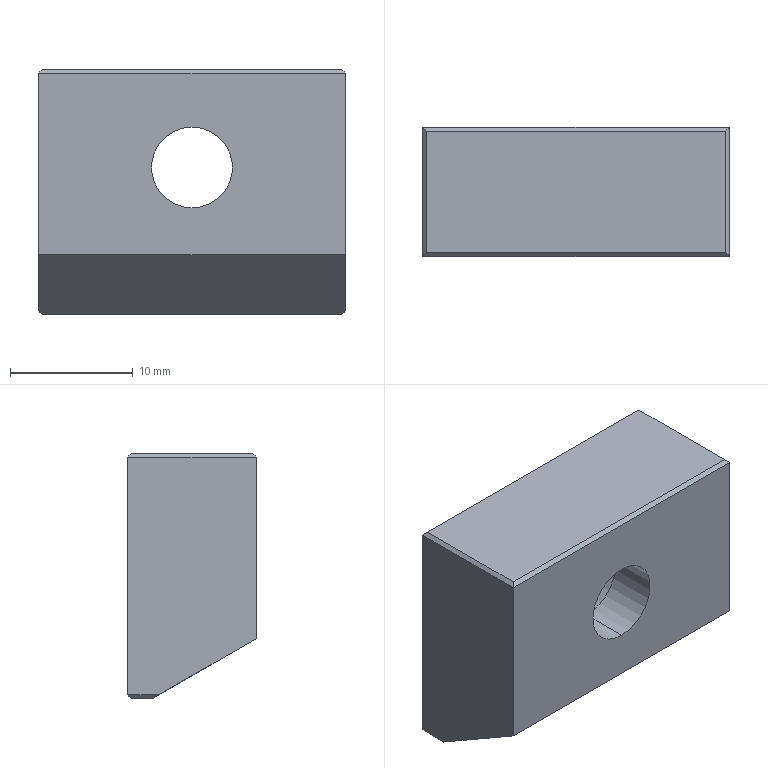Part | STEP file | P-0082091 | 1 solid | 19 faces | box 25 x 10.5 x 20 mm | volume 3970 mm3 | plane 15 | cylinder 4 | commonest cylinder face diameters 6.6 x2 11 x2
STEP:
#1=CARTESIAN_POINT('',(0.,0.,0.));
#2=DIRECTION('',(0.,0.,1.));
#3=DIRECTION('',(1.,0.,0.));
#4=AXIS2_PLACEMENT_3D('',#1,#2,#3);
#5=CARTESIAN_POINT('',(0.,-1.25,7.5));
#6=VERTEX_POINT('',#5);
#7=CARTESIAN_POINT('',(0.,5.25,7.5));
#8=VERTEX_POINT('',#7);
#9=CARTESIAN_POINT('',(0.,5.25,7.5));
#10=DIRECTION('',(0.,1.,0.));
#11=VECTOR('',#10,1.);
#12=LINE('',#9,#11);
#13=CARTESIAN_POINT('',(0.,5.25,2.));
#14=DIRECTION('',(0.,1.,0.));
#15=DIRECTION('',(0.,0.,1.));
#16=AXIS2_PLACEMENT_3D('',#13,#14,#15);
#17=CYLINDRICAL_SURFACE('',#16,5.5);
#18=CARTESIAN_POINT('',(6.283,0.));
#19=DIRECTION('',(0.,1.));
#20=VECTOR('',#19,1.);
#21=LINE('',#18,#20);
#22=(GEOMETRIC_REPRESENTATION_CONTEXT(2)PARAMETRIC_REPRESENTATION_CONTEXT()REPRESENTATION_CONTEXT('',''));
#23=DEFINITIONAL_REPRESENTATION('',(#21),#22);
#24=PCURVE('',#17,#23);
#25=CARTESIAN_POINT('',(0.,5.25,2.));
#26=DIRECTION('',(0.,1.,0.));
#27=DIRECTION('',(0.,0.,1.));
#28=AXIS2_PLACEMENT_3D('',#25,#26,#27);
#29=CYLINDRICAL_SURFACE('',#28,5.5);
#30=CARTESIAN_POINT('',(0.,0.));
#31=DIRECTION('',(0.,1.));
#32=VECTOR('',#31,1.);
#33=LINE('',#30,#32);
#34=(GEOMETRIC_REPRESENTATION_CONTEXT(2)PARAMETRIC_REPRESENTATION_CONTEXT()REPRESENTATION_CONTEXT('',''));
#35=DEFINITIONAL_REPRESENTATION('',(#33),#34);
#36=PCURVE('',#29,#35);
#37=SURFACE_CURVE('',#12,(#24,#36),.PCURVE_S1.);
#38=EDGE_CURVE('',#6,#8,#37,.T.);
#39=ORIENTED_EDGE('',*,*,#38,.T.);
#40=CARTESIAN_POINT('',(0.,5.25,-3.5));
#41=VERTEX_POINT('',#40);
#42=CARTESIAN_POINT('',(0.,5.25,2.));
#43=DIRECTION('',(0.,1.,0.));
#44=DIRECTION('',(0.,0.,1.));
#45=AXIS2_PLACEMENT_3D('',#42,#43,#44);
#46=CIRCLE('',#45,5.5);
#47=CARTESIAN_POINT('',(0.,0.));
#48=DIRECTION('',(1.,0.));
#49=VECTOR('',#48,1.);
#50=LINE('',#47,#49);
#51=(GEOMETRIC_REPRESENTATION_CONTEXT(2)PARAMETRIC_REPRESENTATION_CONTEXT()REPRESENTATION_CONTEXT('',''));
#52=DEFINITIONAL_REPRESENTATION('',(#50),#51);
#53=PCURVE('',#17,#52);
#54=CARTESIAN_POINT('',(12.5,5.25,10.));
#55=DIRECTION('',(0.,-1.,0.));
#56=DIRECTION('',(0.,0.,-1.));
#57=AXIS2_PLACEMENT_3D('',#54,#55,#56);
#58=PLANE('',#57);
#59=CARTESIAN_POINT('',(2.5,-12.5));
#60=CARTESIAN_POINT('',(2.5,-2.974));
#61=CARTESIAN_POINT('',(10.75,-7.737));
#62=CARTESIAN_POINT('',(19.,-12.5));
#63=CARTESIAN_POINT('',(10.75,-17.263));
#64=CARTESIAN_POINT('',(2.5,-22.026));
#65=CARTESIAN_POINT('',(2.5,-12.5));
#66=(BOUNDED_CURVE()B_SPLINE_CURVE(2,(#59,#60,#61,#62,#63,#64,#65),.UNSPECIFIED.,.T.,.F.)B_SPLINE_CURVE_WITH_KNOTS((1,2,2,2,2,1),(-2.094,0.,2.094,4.189,6.283,8.378),.UNSPECIFIED.)CURVE()GEOMETRIC_REPRESENTATION_ITEM()RATIONAL_B_SPLINE_CURVE((1.,0.5,1.,0.5,1.,0.5,1.))REPRESENTATION_ITEM(''));
#67=(GEOMETRIC_REPRESENTATION_CONTEXT(2)PARAMETRIC_REPRESENTATION_CONTEXT()REPRESENTATION_CONTEXT('',''));
#68=DEFINITIONAL_REPRESENTATION('',(#66),#67);
#69=PCURVE('',#58,#68);
#70=SURFACE_CURVE('',#46,(#53,#69),.PCURVE_S1.);
#71=EDGE_CURVE('',#41,#8,#70,.T.);
#72=ORIENTED_EDGE('',*,*,#71,.F.);
#73=CARTESIAN_POINT('',(0.,-1.25,-3.5));
#74=VERTEX_POINT('',#73);
#75=CARTESIAN_POINT('',(0.,5.25,-3.5));
#76=DIRECTION('',(0.,1.,0.));
#77=VECTOR('',#76,1.);
#78=LINE('',#75,#77);
#79=CARTESIAN_POINT('',(3.142,0.));
#80=DIRECTION('',(0.,1.));
#81=VECTOR('',#80,1.);
#82=LINE('',#79,#81);
#83=(GEOMETRIC_REPRESENTATION_CONTEXT(2)PARAMETRIC_REPRESENTATION_CONTEXT()REPRESENTATION_CONTEXT('',''));
#84=DEFINITIONAL_REPRESENTATION('',(#82),#83);
#85=PCURVE('',#17,#84);
#86=CARTESIAN_POINT('',(3.142,0.));
#87=DIRECTION('',(0.,1.));
#88=VECTOR('',#87,1.);
#89=LINE('',#86,#88);
#90=(GEOMETRIC_REPRESENTATION_CONTEXT(2)PARAMETRIC_REPRESENTATION_CONTEXT()REPRESENTATION_CONTEXT('',''));
#91=DEFINITIONAL_REPRESENTATION('',(#89),#90);
#92=PCURVE('',#29,#91);
#93=SURFACE_CURVE('',#78,(#85,#92),.PCURVE_S1.);
#94=EDGE_CURVE('',#74,#41,#93,.T.);
#95=ORIENTED_EDGE('',*,*,#94,.F.);
#96=CARTESIAN_POINT('',(0.,-1.25,2.));
#97=DIRECTION('',(0.,1.,0.));
#98=DIRECTION('',(0.,0.,1.));
#99=AXIS2_PLACEMENT_3D('',#96,#97,#98);
#100=CIRCLE('',#99,5.5);
#101=CARTESIAN_POINT('',(0.,-6.5));
#102=DIRECTION('',(1.,0.));
#103=VECTOR('',#102,1.);
#104=LINE('',#101,#103);
#105=(GEOMETRIC_REPRESENTATION_CONTEXT(2)PARAMETRIC_REPRESENTATION_CONTEXT()REPRESENTATION_CONTEXT('',''));
#106=DEFINITIONAL_REPRESENTATION('',(#104),#105);
#107=PCURVE('',#17,#106);
#108=CARTESIAN_POINT('',(3.3,-1.25,2.));
#109=DIRECTION('',(0.,-1.,0.));
#110=DIRECTION('',(0.,0.,-1.));
#111=AXIS2_PLACEMENT_3D('',#108,#109,#110);
#112=PLANE('',#111);
#113=CARTESIAN_POINT('',(-5.5,-3.3));
#114=CARTESIAN_POINT('',(-5.5,6.226));
#115=CARTESIAN_POINT('',(2.75,1.463));
#116=CARTESIAN_POINT('',(11.,-3.3));
#117=CARTESIAN_POINT('',(2.75,-8.063));
#118=CARTESIAN_POINT('',(-5.5,-12.826));
#119=CARTESIAN_POINT('',(-5.5,-3.3));
#120=(BOUNDED_CURVE()B_SPLINE_CURVE(2,(#113,#114,#115,#116,#117,#118,#119),.UNSPECIFIED.,.T.,.F.)B_SPLINE_CURVE_WITH_KNOTS((1,2,2,2,2,1),(-2.094,0.,2.094,4.189,6.283,8.378),.UNSPECIFIED.)CURVE()GEOMETRIC_REPRESENTATION_ITEM()RATIONAL_B_SPLINE_CURVE((1.,0.5,1.,0.5,1.,0.5,1.))REPRESENTATION_ITEM(''));
#121=(GEOMETRIC_REPRESENTATION_CONTEXT(2)PARAMETRIC_REPRESENTATION_CONTEXT()REPRESENTATION_CONTEXT('',''));
#122=DEFINITIONAL_REPRESENTATION('',(#120),#121);
#123=PCURVE('',#112,#122);
#124=SURFACE_CURVE('',#100,(#107,#123),.PCURVE_S1.);
#125=EDGE_CURVE('',#74,#6,#124,.T.);
#126=ORIENTED_EDGE('',*,*,#125,.T.);
#127=EDGE_LOOP('',(#39,#72,#95,#126));
#128=FACE_BOUND('',#127,.F.);
#129=ADVANCED_FACE('',(#128),#17,.F.);
#130=CARTESIAN_POINT('',(0.,-5.25,5.3));
#131=VERTEX_POINT('',#130);
#132=CARTESIAN_POINT('',(0.,-1.25,5.3));
#133=VERTEX_POINT('',#132);
#134=CARTESIAN_POINT('',(0.,5.25,5.3));
#135=DIRECTION('',(0.,1.,0.));
#136=VECTOR('',#135,1.);
#137=LINE('',#134,#136);
#138=CARTESIAN_POINT('',(0.,5.25,2.));
#139=DIRECTION('',(0.,1.,0.));
#140=DIRECTION('',(0.,0.,1.));
#141=AXIS2_PLACEMENT_3D('',#138,#139,#140);
#142=CYLINDRICAL_SURFACE('',#141,3.3);
#143=CARTESIAN_POINT('',(6.283,0.));
#144=DIRECTION('',(0.,1.));
#145=VECTOR('',#144,1.);
#146=LINE('',#143,#145);
#147=(GEOMETRIC_REPRESENTATION_CONTEXT(2)PARAMETRIC_REPRESENTATION_CONTEXT()REPRESENTATION_CONTEXT('',''));
#148=DEFINITIONAL_REPRESENTATION('',(#146),#147);
#149=PCURVE('',#142,#148);
#150=CARTESIAN_POINT('',(0.,5.25,2.));
#151=DIRECTION('',(0.,1.,0.));
#152=DIRECTION('',(0.,0.,1.));
#153=AXIS2_PLACEMENT_3D('',#150,#151,#152);
#154=CYLINDRICAL_SURFACE('',#153,3.3);
#155=CARTESIAN_POINT('',(0.,0.));
#156=DIRECTION('',(0.,1.));
#157=VECTOR('',#156,1.);
#158=LINE('',#155,#157);
#159=(GEOMETRIC_REPRESENTATION_CONTEXT(2)PARAMETRIC_REPRESENTATION_CONTEXT()REPRESENTATION_CONTEXT('',''));
#160=DEFINITIONAL_REPRESENTATION('',(#158),#159);
#161=PCURVE('',#154,#160);
#162=SURFACE_CURVE('',#137,(#149,#161),.PCURVE_S1.);
#163=EDGE_CURVE('',#131,#133,#162,.T.);
#164=ORIENTED_EDGE('',*,*,#163,.T.);
#165=CARTESIAN_POINT('',(0.,-1.25,-1.3));
#166=VERTEX_POINT('',#165);
#167=CARTESIAN_POINT('',(0.,-1.25,2.));
#168=DIRECTION('',(0.,1.,0.));
#169=DIRECTION('',(0.,0.,1.));
#170=AXIS2_PLACEMENT_3D('',#167,#168,#169);
#171=CIRCLE('',#170,3.3);
#172=CARTESIAN_POINT('',(0.,-6.5));
#173=DIRECTION('',(1.,0.));
#174=VECTOR('',#173,1.);
#175=LINE('',#172,#174);
#176=(GEOMETRIC_REPRESENTATION_CONTEXT(2)PARAMETRIC_REPRESENTATION_CONTEXT()REPRESENTATION_CONTEXT('',''));
#177=DEFINITIONAL_REPRESENTATION('',(#175),#176);
#178=PCURVE('',#142,#177);
#179=CARTESIAN_POINT('',(-3.3,-3.3));
#180=CARTESIAN_POINT('',(-3.3,2.416));
#181=CARTESIAN_POINT('',(1.65,-0.4421));
#182=CARTESIAN_POINT('',(6.6,-3.3));
#183=CARTESIAN_POINT('',(1.65,-6.158));
#184=CARTESIAN_POINT('',(-3.3,-9.016));
#185=CARTESIAN_POINT('',(-3.3,-3.3));
#186=(BOUNDED_CURVE()B_SPLINE_CURVE(2,(#179,#180,#181,#182,#183,#184,#185),.UNSPECIFIED.,.T.,.F.)B_SPLINE_CURVE_WITH_KNOTS((1,2,2,2,2,1),(-2.094,0.,2.094,4.189,6.283,8.378),.UNSPECIFIED.)CURVE()GEOMETRIC_REPRESENTATION_ITEM()RATIONAL_B_SPLINE_CURVE((1.,0.5,1.,0.5,1.,0.5,1.))REPRESENTATION_ITEM(''));
#187=(GEOMETRIC_REPRESENTATION_CONTEXT(2)PARAMETRIC_REPRESENTATION_CONTEXT()REPRESENTATION_CONTEXT('',''));
#188=DEFINITIONAL_REPRESENTATION('',(#186),#187);
#189=PCURVE('',#112,#188);
#190=SURFACE_CURVE('',#171,(#178,#189),.PCURVE_S1.);
#191=EDGE_CURVE('',#166,#133,#190,.T.);
#192=ORIENTED_EDGE('',*,*,#191,.F.);
#193=CARTESIAN_POINT('',(0.,-5.25,-1.3));
#194=VERTEX_POINT('',#193);
#195=CARTESIAN_POINT('',(0.,5.25,-1.3));
#196=DIRECTION('',(0.,1.,0.));
#197=VECTOR('',#196,1.);
#198=LINE('',#195,#197);
#199=CARTESIAN_POINT('',(3.142,0.));
#200=DIRECTION('',(0.,1.));
#201=VECTOR('',#200,1.);
#202=LINE('',#199,#201);
#203=(GEOMETRIC_REPRESENTATION_CONTEXT(2)PARAMETRIC_REPRESENTATION_CONTEXT()REPRESENTATION_CONTEXT('',''));
#204=DEFINITIONAL_REPRESENTATION('',(#202),#203);
#205=PCURVE('',#142,#204);
#206=CARTESIAN_POINT('',(3.142,0.));
#207=DIRECTION('',(0.,1.));
#208=VECTOR('',#207,1.);
#209=LINE('',#206,#208);
#210=(GEOMETRIC_REPRESENTATION_CONTEXT(2)PARAMETRIC_REPRESENTATION_CONTEXT()REPRESENTATION_CONTEXT('',''));
#211=DEFINITIONAL_REPRESENTATION('',(#209),#210);
#212=PCURVE('',#154,#211);
#213=SURFACE_CURVE('',#198,(#205,#212),.PCURVE_S1.);
#214=EDGE_CURVE('',#194,#166,#213,.T.);
#215=ORIENTED_EDGE('',*,*,#214,.F.);
#216=CARTESIAN_POINT('',(0.,-5.25,2.));
#217=DIRECTION('',(0.,1.,0.));
#218=DIRECTION('',(0.,0.,1.));
#219=AXIS2_PLACEMENT_3D('',#216,#217,#218);
#220=CIRCLE('',#219,3.3);
#221=CARTESIAN_POINT('',(0.,-10.5));
#222=DIRECTION('',(1.,0.));
#223=VECTOR('',#222,1.);
#224=LINE('',#221,#223);
#225=(GEOMETRIC_REPRESENTATION_CONTEXT(2)PARAMETRIC_REPRESENTATION_CONTEXT()REPRESENTATION_CONTEXT('',''));
#226=DEFINITIONAL_REPRESENTATION('',(#224),#225);
#227=PCURVE('',#142,#226);
#228=CARTESIAN_POINT('',(12.5,-5.25,-5.1));
#229=DIRECTION('',(0.,1.,0.));
#230=DIRECTION('',(0.,0.,1.));
#231=AXIS2_PLACEMENT_3D('',#228,#229,#230);
#232=PLANE('',#231);
#233=CARTESIAN_POINT('',(7.1,-12.5));
#234=DIRECTION('',(1.,0.));
#235=AXIS2_PLACEMENT_2D('',#233,#234);
#236=CIRCLE('',#235,3.3);
#237=(GEOMETRIC_REPRESENTATION_CONTEXT(2)PARAMETRIC_REPRESENTATION_CONTEXT()REPRESENTATION_CONTEXT('',''));
#238=DEFINITIONAL_REPRESENTATION('',(#236),#237);
#239=PCURVE('',#232,#238);
#240=SURFACE_CURVE('',#220,(#227,#239),.PCURVE_S1.);
#241=EDGE_CURVE('',#194,#131,#240,.T.);
#242=ORIENTED_EDGE('',*,*,#241,.T.);
#243=EDGE_LOOP('',(#164,#192,#215,#242));
#244=FACE_BOUND('',#243,.F.);
#245=ADVANCED_FACE('',(#244),#142,.F.);
#246=CARTESIAN_POINT('',(0.,-5.25,2.));
#247=DIRECTION('',(0.,1.,0.));
#248=DIRECTION('',(0.,0.,1.));
#249=AXIS2_PLACEMENT_3D('',#246,#247,#248);
#250=CIRCLE('',#249,3.3);
#251=CARTESIAN_POINT('',(7.1,-12.5));
#252=DIRECTION('',(1.,0.));
#253=AXIS2_PLACEMENT_2D('',#251,#252);
#254=CIRCLE('',#253,3.3);
#255=(GEOMETRIC_REPRESENTATION_CONTEXT(2)PARAMETRIC_REPRESENTATION_CONTEXT()REPRESENTATION_CONTEXT('',''));
#256=DEFINITIONAL_REPRESENTATION('',(#254),#255);
#257=PCURVE('',#232,#256);
#258=CARTESIAN_POINT('',(0.,-10.5));
#259=DIRECTION('',(1.,0.));
#260=VECTOR('',#259,1.);
#261=LINE('',#258,#260);
#262=(GEOMETRIC_REPRESENTATION_CONTEXT(2)PARAMETRIC_REPRESENTATION_CONTEXT()REPRESENTATION_CONTEXT('',''));
#263=DEFINITIONAL_REPRESENTATION('',(#261),#262);
#264=PCURVE('',#154,#263);
#265=SURFACE_CURVE('',#250,(#257,#264),.PCURVE_S1.);
#266=EDGE_CURVE('',#131,#194,#265,.T.);
#267=ORIENTED_EDGE('',*,*,#266,.T.);
#268=ORIENTED_EDGE('',*,*,#241,.T.);
#269=EDGE_LOOP('',(#267,#268));
#270=FACE_BOUND('',#269,.T.);
#271=CARTESIAN_POINT('',(12.5,-5.25,9.7));
#272=VERTEX_POINT('',#271);
#273=CARTESIAN_POINT('',(12.5,-5.25,-5.1));
#274=VERTEX_POINT('',#273);
#275=CARTESIAN_POINT('',(12.5,-5.25,-5.1));
#276=DIRECTION('',(0.,0.,-1.));
#277=VECTOR('',#276,1.);
#278=LINE('',#275,#277);
#279=CARTESIAN_POINT('',(0.,0.));
#280=DIRECTION('',(-1.,0.));
#281=VECTOR('',#280,1.);
#282=LINE('',#279,#281);
#283=(GEOMETRIC_REPRESENTATION_CONTEXT(2)PARAMETRIC_REPRESENTATION_CONTEXT()REPRESENTATION_CONTEXT('',''));
#284=DEFINITIONAL_REPRESENTATION('',(#282),#283);
#285=PCURVE('',#232,#284);
#286=CARTESIAN_POINT('',(12.5,0.,0.));
#287=DIRECTION('',(-1.,0.,0.));
#288=DIRECTION('',(0.,0.,1.));
#289=AXIS2_PLACEMENT_3D('',#286,#287,#288);
#290=PLANE('',#289);
#291=CARTESIAN_POINT('',(-5.1,-5.25));
#292=DIRECTION('',(-1.,0.));
#293=VECTOR('',#292,1.);
#294=LINE('',#291,#293);
#295=(GEOMETRIC_REPRESENTATION_CONTEXT(2)PARAMETRIC_REPRESENTATION_CONTEXT()REPRESENTATION_CONTEXT('',''));
#296=DEFINITIONAL_REPRESENTATION('',(#294),#295);
#297=PCURVE('',#290,#296);
#298=SURFACE_CURVE('',#278,(#285,#297),.PCURVE_S1.);
#299=EDGE_CURVE('',#272,#274,#298,.T.);
#300=ORIENTED_EDGE('',*,*,#299,.F.);
#301=CARTESIAN_POINT('',(-12.5,-5.25,9.7));
#302=VERTEX_POINT('',#301);
#303=CARTESIAN_POINT('',(12.5,-5.25,9.7));
#304=DIRECTION('',(-1.,0.,0.));
#305=VECTOR('',#304,1.);
#306=LINE('',#303,#305);
#307=CARTESIAN_POINT('',(14.8,0.));
#308=DIRECTION('',(0.,-1.));
#309=VECTOR('',#308,1.);
#310=LINE('',#307,#309);
#311=(GEOMETRIC_REPRESENTATION_CONTEXT(2)PARAMETRIC_REPRESENTATION_CONTEXT()REPRESENTATION_CONTEXT('',''));
#312=DEFINITIONAL_REPRESENTATION('',(#310),#311);
#313=PCURVE('',#232,#312);
#314=CARTESIAN_POINT('',(12.5,-5.25,9.7));
#315=DIRECTION('',(0.,0.7071,-0.7071));
#316=DIRECTION('',(-1.,0.,0.));
#317=AXIS2_PLACEMENT_3D('',#314,#315,#316);
#318=PLANE('',#317);
#319=CARTESIAN_POINT('',(0.,0.));
#320=DIRECTION('',(1.,0.));
#321=VECTOR('',#320,1.);
#322=LINE('',#319,#321);
#323=(GEOMETRIC_REPRESENTATION_CONTEXT(2)PARAMETRIC_REPRESENTATION_CONTEXT()REPRESENTATION_CONTEXT('',''));
#324=DEFINITIONAL_REPRESENTATION('',(#322),#323);
#325=PCURVE('',#318,#324);
#326=SURFACE_CURVE('',#306,(#313,#325),.PCURVE_S1.);
#327=EDGE_CURVE('',#272,#302,#326,.T.);
#328=ORIENTED_EDGE('',*,*,#327,.T.);
#329=CARTESIAN_POINT('',(-12.5,-5.25,-5.1));
#330=VERTEX_POINT('',#329);
#331=CARTESIAN_POINT('',(-12.5,-5.25,-5.1));
#332=DIRECTION('',(0.,0.,-1.));
#333=VECTOR('',#332,1.);
#334=LINE('',#331,#333);
#335=CARTESIAN_POINT('',(0.,-25.));
#336=DIRECTION('',(-1.,0.));
#337=VECTOR('',#336,1.);
#338=LINE('',#335,#337);
#339=(GEOMETRIC_REPRESENTATION_CONTEXT(2)PARAMETRIC_REPRESENTATION_CONTEXT()REPRESENTATION_CONTEXT('',''));
#340=DEFINITIONAL_REPRESENTATION('',(#338),#339);
#341=PCURVE('',#232,#340);
#342=CARTESIAN_POINT('',(-12.5,0.,0.));
#343=DIRECTION('',(-1.,0.,0.));
#344=DIRECTION('',(0.,0.,1.));
#345=AXIS2_PLACEMENT_3D('',#342,#343,#344);
#346=PLANE('',#345);
#347=CARTESIAN_POINT('',(-5.1,-5.25));
#348=DIRECTION('',(-1.,0.));
#349=VECTOR('',#348,1.);
#350=LINE('',#347,#349);
#351=(GEOMETRIC_REPRESENTATION_CONTEXT(2)PARAMETRIC_REPRESENTATION_CONTEXT()REPRESENTATION_CONTEXT('',''));
#352=DEFINITIONAL_REPRESENTATION('',(#350),#351);
#353=PCURVE('',#346,#352);
#354=SURFACE_CURVE('',#334,(#341,#353),.PCURVE_S1.);
#355=EDGE_CURVE('',#302,#330,#354,.T.);
#356=ORIENTED_EDGE('',*,*,#355,.T.);
#357=CARTESIAN_POINT('',(12.5,-5.25,-5.1));
#358=DIRECTION('',(-1.,0.,0.));
#359=VECTOR('',#358,1.);
#360=LINE('',#357,#359);
#361=CARTESIAN_POINT('',(0.,0.));
#362=DIRECTION('',(0.,-1.));
#363=VECTOR('',#362,1.);
#364=LINE('',#361,#363);
#365=(GEOMETRIC_REPRESENTATION_CONTEXT(2)PARAMETRIC_REPRESENTATION_CONTEXT()REPRESENTATION_CONTEXT('',''));
#366=DEFINITIONAL_REPRESENTATION('',(#364),#365);
#367=PCURVE('',#232,#366);
#368=CARTESIAN_POINT('',(12.5,3.25,-10.));
#369=DIRECTION('',(0.,0.4994,0.8664));
#370=DIRECTION('',(0.,-0.8664,0.4994));
#371=AXIS2_PLACEMENT_3D('',#368,#369,#370);
#372=PLANE('',#371);
#373=CARTESIAN_POINT('',(9.811,0.));
#374=DIRECTION('',(0.,-1.));
#375=VECTOR('',#374,1.);
#376=LINE('',#373,#375);
#377=(GEOMETRIC_REPRESENTATION_CONTEXT(2)PARAMETRIC_REPRESENTATION_CONTEXT()REPRESENTATION_CONTEXT('',''));
#378=DEFINITIONAL_REPRESENTATION('',(#376),#377);
#379=PCURVE('',#372,#378);
#380=SURFACE_CURVE('',#360,(#367,#379),.PCURVE_S1.);
#381=EDGE_CURVE('',#274,#330,#380,.T.);
#382=ORIENTED_EDGE('',*,*,#381,.F.);
#383=EDGE_LOOP('',(#300,#328,#356,#382));
#384=FACE_BOUND('',#383,.T.);
#385=ADVANCED_FACE('',(#270,#384),#232,.F.);
#386=CARTESIAN_POINT('',(-12.5,2.73,-9.7));
#387=VERTEX_POINT('',#386);
#388=CARTESIAN_POINT('',(-12.5,3.25,-10.));
#389=DIRECTION('',(0.,0.8664,-0.4994));
#390=VECTOR('',#389,1.);
#391=LINE('',#388,#390);
#392=CARTESIAN_POINT('',(0.,-25.));
#393=DIRECTION('',(-1.,0.));
#394=VECTOR('',#393,1.);
#395=LINE('',#392,#394);
#396=(GEOMETRIC_REPRESENTATION_CONTEXT(2)PARAMETRIC_REPRESENTATION_CONTEXT()REPRESENTATION_CONTEXT('',''));
#397=DEFINITIONAL_REPRESENTATION('',(#395),#396);
#398=PCURVE('',#372,#397);
#399=CARTESIAN_POINT('',(-10.,3.25));
#400=DIRECTION('',(-0.4994,0.8664));
#401=VECTOR('',#400,1.);
#402=LINE('',#399,#401);
#403=(GEOMETRIC_REPRESENTATION_CONTEXT(2)PARAMETRIC_REPRESENTATION_CONTEXT()REPRESENTATION_CONTEXT('',''));
#404=DEFINITIONAL_REPRESENTATION('',(#402),#403);
#405=PCURVE('',#346,#404);
#406=SURFACE_CURVE('',#391,(#398,#405),.PCURVE_S1.);
#407=EDGE_CURVE('',#330,#387,#406,.T.);
#408=ORIENTED_EDGE('',*,*,#407,.T.);
#409=CARTESIAN_POINT('',(-12.2,3.25,-10.));
#410=VERTEX_POINT('',#409);
#411=CARTESIAN_POINT('',(-11.507,4.451,-10.693));
#412=DIRECTION('',(0.4468,0.7751,-0.4468));
#413=VECTOR('',#412,1.);
#414=LINE('',#411,#413);
#415=CARTESIAN_POINT('',(-1.387,-24.007));
#416=DIRECTION('',(-0.8946,0.4468));
#417=VECTOR('',#416,1.);
#418=LINE('',#415,#417);
#419=(GEOMETRIC_REPRESENTATION_CONTEXT(2)PARAMETRIC_REPRESENTATION_CONTEXT()REPRESENTATION_CONTEXT('',''));
#420=DEFINITIONAL_REPRESENTATION('',(#418),#419);
#421=PCURVE('',#372,#420);
#422=CARTESIAN_POINT('',(-12.2,5.25,-10.));
#423=DIRECTION('',(-0.7071,0.,-0.7071));
#424=DIRECTION('',(0.,-1.,0.));
#425=AXIS2_PLACEMENT_3D('',#422,#423,#424);
#426=PLANE('',#425);
#427=CARTESIAN_POINT('',(0.7985,-0.9795));
#428=DIRECTION('',(-0.7751,-0.6319));
#429=VECTOR('',#428,1.);
#430=LINE('',#427,#429);
#431=(GEOMETRIC_REPRESENTATION_CONTEXT(2)PARAMETRIC_REPRESENTATION_CONTEXT()REPRESENTATION_CONTEXT('',''));
#432=DEFINITIONAL_REPRESENTATION('',(#430),#431);
#433=PCURVE('',#426,#432);
#434=SURFACE_CURVE('',#414,(#421,#433),.PCURVE_S1.);
#435=EDGE_CURVE('',#387,#410,#434,.T.);
#436=ORIENTED_EDGE('',*,*,#435,.T.);
#437=CARTESIAN_POINT('',(12.2,3.25,-10.));
#438=VERTEX_POINT('',#437);
#439=CARTESIAN_POINT('',(12.5,3.25,-10.));
#440=DIRECTION('',(-1.,0.,0.));
#441=VECTOR('',#440,1.);
#442=LINE('',#439,#441);
#443=CARTESIAN_POINT('',(0.,0.));
#444=DIRECTION('',(0.,-1.));
#445=VECTOR('',#444,1.);
#446=LINE('',#443,#445);
#447=(GEOMETRIC_REPRESENTATION_CONTEXT(2)PARAMETRIC_REPRESENTATION_CONTEXT()REPRESENTATION_CONTEXT('',''));
#448=DEFINITIONAL_REPRESENTATION('',(#446),#447);
#449=PCURVE('',#372,#448);
#450=CARTESIAN_POINT('',(12.5,5.25,-10.));
#451=DIRECTION('',(0.,0.,1.));
#452=DIRECTION('',(1.,0.,0.));
#453=AXIS2_PLACEMENT_3D('',#450,#451,#452);
#454=PLANE('',#453);
#455=CARTESIAN_POINT('',(0.,-2.));
#456=DIRECTION('',(-1.,0.));
#457=VECTOR('',#456,1.);
#458=LINE('',#455,#457);
#459=(GEOMETRIC_REPRESENTATION_CONTEXT(2)PARAMETRIC_REPRESENTATION_CONTEXT()REPRESENTATION_CONTEXT('',''));
#460=DEFINITIONAL_REPRESENTATION('',(#458),#459);
#461=PCURVE('',#454,#460);
#462=SURFACE_CURVE('',#442,(#449,#461),.PCURVE_S1.);
#463=EDGE_CURVE('',#438,#410,#462,.T.);
#464=ORIENTED_EDGE('',*,*,#463,.F.);
#465=CARTESIAN_POINT('',(12.5,2.73,-9.7));
#466=VERTEX_POINT('',#465);
#467=CARTESIAN_POINT('',(13.445,1.09,-8.755));
#468=DIRECTION('',(0.4468,-0.7751,0.4468));
#469=VECTOR('',#468,1.);
#470=LINE('',#467,#469);
#471=CARTESIAN_POINT('',(2.493,0.9453));
#472=DIRECTION('',(0.8946,0.4468));
#473=VECTOR('',#472,1.);
#474=LINE('',#471,#473);
#475=(GEOMETRIC_REPRESENTATION_CONTEXT(2)PARAMETRIC_REPRESENTATION_CONTEXT()REPRESENTATION_CONTEXT('',''));
#476=DEFINITIONAL_REPRESENTATION('',(#474),#475);
#477=PCURVE('',#372,#476);
#478=CARTESIAN_POINT('',(12.5,0.,-9.7));
#479=DIRECTION('',(-0.7071,0.,0.7071));
#480=DIRECTION('',(0.,1.,0.));
#481=AXIS2_PLACEMENT_3D('',#478,#479,#480);
#482=PLANE('',#481);
#483=CARTESIAN_POINT('',(1.09,-1.337));
#484=DIRECTION('',(-0.7751,-0.6319));
#485=VECTOR('',#484,1.);
#486=LINE('',#483,#485);
#487=(GEOMETRIC_REPRESENTATION_CONTEXT(2)PARAMETRIC_REPRESENTATION_CONTEXT()REPRESENTATION_CONTEXT('',''));
#488=DEFINITIONAL_REPRESENTATION('',(#486),#487);
#489=PCURVE('',#482,#488);
#490=SURFACE_CURVE('',#470,(#477,#489),.PCURVE_S1.);
#491=EDGE_CURVE('',#438,#466,#490,.T.);
#492=ORIENTED_EDGE('',*,*,#491,.T.);
#493=CARTESIAN_POINT('',(12.5,3.25,-10.));
#494=DIRECTION('',(0.,0.8664,-0.4994));
#495=VECTOR('',#494,1.);
#496=LINE('',#493,#495);
#497=CARTESIAN_POINT('',(0.,0.));
#498=DIRECTION('',(-1.,0.));
#499=VECTOR('',#498,1.);
#500=LINE('',#497,#499);
#501=(GEOMETRIC_REPRESENTATION_CONTEXT(2)PARAMETRIC_REPRESENTATION_CONTEXT()REPRESENTATION_CONTEXT('',''));
#502=DEFINITIONAL_REPRESENTATION('',(#500),#501);
#503=PCURVE('',#372,#502);
#504=CARTESIAN_POINT('',(-10.,3.25));
#505=DIRECTION('',(-0.4994,0.8664));
#506=VECTOR('',#505,1.);
#507=LINE('',#504,#506);
#508=(GEOMETRIC_REPRESENTATION_CONTEXT(2)PARAMETRIC_REPRESENTATION_CONTEXT()REPRESENTATION_CONTEXT('',''));
#509=DEFINITIONAL_REPRESENTATION('',(#507),#508);
#510=PCURVE('',#290,#509);
#511=SURFACE_CURVE('',#496,(#503,#510),.PCURVE_S1.);
#512=EDGE_CURVE('',#274,#466,#511,.T.);
#513=ORIENTED_EDGE('',*,*,#512,.F.);
#514=ORIENTED_EDGE('',*,*,#381,.T.);
#515=EDGE_LOOP('',(#408,#436,#464,#492,#513,#514));
#516=FACE_BOUND('',#515,.T.);
#517=ADVANCED_FACE('',(#516),#372,.F.);
#518=ORIENTED_EDGE('',*,*,#463,.T.);
#519=CARTESIAN_POINT('',(-12.2,4.95,-10.));
#520=VERTEX_POINT('',#519);
#521=CARTESIAN_POINT('',(-12.2,5.25,-10.));
#522=DIRECTION('',(0.,1.,0.));
#523=VECTOR('',#522,1.);
#524=LINE('',#521,#523);
#525=CARTESIAN_POINT('',(-24.7,0.));
#526=DIRECTION('',(0.,1.));
#527=VECTOR('',#526,1.);
#528=LINE('',#525,#527);
#529=(GEOMETRIC_REPRESENTATION_CONTEXT(2)PARAMETRIC_REPRESENTATION_CONTEXT()REPRESENTATION_CONTEXT('',''));
#530=DEFINITIONAL_REPRESENTATION('',(#528),#529);
#531=PCURVE('',#454,#530);
#532=CARTESIAN_POINT('',(0.,0.));
#533=DIRECTION('',(-1.,0.));
#534=VECTOR('',#533,1.);
#535=LINE('',#532,#534);
#536=(GEOMETRIC_REPRESENTATION_CONTEXT(2)PARAMETRIC_REPRESENTATION_CONTEXT()REPRESENTATION_CONTEXT('',''));
#537=DEFINITIONAL_REPRESENTATION('',(#535),#536);
#538=PCURVE('',#426,#537);
#539=SURFACE_CURVE('',#524,(#531,#538),.PCURVE_S1.);
#540=EDGE_CURVE('',#410,#520,#539,.T.);
#541=ORIENTED_EDGE('',*,*,#540,.T.);
#542=CARTESIAN_POINT('',(12.2,4.95,-10.));
#543=VERTEX_POINT('',#542);
#544=CARTESIAN_POINT('',(12.5,4.95,-10.));
#545=DIRECTION('',(1.,0.,0.));
#546=VECTOR('',#545,1.);
#547=LINE('',#544,#546);
#548=CARTESIAN_POINT('',(0.,-0.3));
#549=DIRECTION('',(1.,0.));
#550=VECTOR('',#549,1.);
#551=LINE('',#548,#550);
#552=(GEOMETRIC_REPRESENTATION_CONTEXT(2)PARAMETRIC_REPRESENTATION_CONTEXT()REPRESENTATION_CONTEXT('',''));
#553=DEFINITIONAL_REPRESENTATION('',(#551),#552);
#554=PCURVE('',#454,#553);
#555=CARTESIAN_POINT('',(12.5,5.25,-9.7));
#556=DIRECTION('',(0.,-0.7071,0.7071));
#557=DIRECTION('',(-1.,0.,0.));
#558=AXIS2_PLACEMENT_3D('',#555,#556,#557);
#559=PLANE('',#558);
#560=CARTESIAN_POINT('',(0.,0.4243));
#561=DIRECTION('',(-1.,0.));
#562=VECTOR('',#561,1.);
#563=LINE('',#560,#562);
#564=(GEOMETRIC_REPRESENTATION_CONTEXT(2)PARAMETRIC_REPRESENTATION_CONTEXT()REPRESENTATION_CONTEXT('',''));
#565=DEFINITIONAL_REPRESENTATION('',(#563),#564);
#566=PCURVE('',#559,#565);
#567=SURFACE_CURVE('',#547,(#554,#566),.PCURVE_S1.);
#568=EDGE_CURVE('',#520,#543,#567,.T.);
#569=ORIENTED_EDGE('',*,*,#568,.T.);
#570=CARTESIAN_POINT('',(12.2,5.25,-10.));
#571=DIRECTION('',(0.,-1.,0.));
#572=VECTOR('',#571,1.);
#573=LINE('',#570,#572);
#574=CARTESIAN_POINT('',(-0.3,0.));
#575=DIRECTION('',(0.,-1.));
#576=VECTOR('',#575,1.);
#577=LINE('',#574,#576);
#578=(GEOMETRIC_REPRESENTATION_CONTEXT(2)PARAMETRIC_REPRESENTATION_CONTEXT()REPRESENTATION_CONTEXT('',''));
#579=DEFINITIONAL_REPRESENTATION('',(#577),#578);
#580=PCURVE('',#454,#579);
#581=CARTESIAN_POINT('',(5.25,0.4243));
#582=DIRECTION('',(-1.,0.));
#583=VECTOR('',#582,1.);
#584=LINE('',#581,#583);
#585=(GEOMETRIC_REPRESENTATION_CONTEXT(2)PARAMETRIC_REPRESENTATION_CONTEXT()REPRESENTATION_CONTEXT('',''));
#586=DEFINITIONAL_REPRESENTATION('',(#584),#585);
#587=PCURVE('',#482,#586);
#588=SURFACE_CURVE('',#573,(#580,#587),.PCURVE_S1.);
#589=EDGE_CURVE('',#543,#438,#588,.T.);
#590=ORIENTED_EDGE('',*,*,#589,.T.);
#591=EDGE_LOOP('',(#518,#541,#569,#590));
#592=FACE_BOUND('',#591,.T.);
#593=ADVANCED_FACE('',(#592),#454,.F.);
#594=CARTESIAN_POINT('',(0.,5.25,2.));
#595=DIRECTION('',(0.,1.,0.));
#596=DIRECTION('',(0.,0.,1.));
#597=AXIS2_PLACEMENT_3D('',#594,#595,#596);
#598=CIRCLE('',#597,5.5);
#599=CARTESIAN_POINT('',(2.5,-12.5));
#600=CARTESIAN_POINT('',(2.5,-2.974));
#601=CARTESIAN_POINT('',(10.75,-7.737));
#602=CARTESIAN_POINT('',(19.,-12.5));
#603=CARTESIAN_POINT('',(10.75,-17.263));
#604=CARTESIAN_POINT('',(2.5,-22.026));
#605=CARTESIAN_POINT('',(2.5,-12.5));
#606=(BOUNDED_CURVE()B_SPLINE_CURVE(2,(#599,#600,#601,#602,#603,#604,#605),.UNSPECIFIED.,.T.,.F.)B_SPLINE_CURVE_WITH_KNOTS((1,2,2,2,2,1),(-2.094,0.,2.094,4.189,6.283,8.378),.UNSPECIFIED.)CURVE()GEOMETRIC_REPRESENTATION_ITEM()RATIONAL_B_SPLINE_CURVE((1.,0.5,1.,0.5,1.,0.5,1.))REPRESENTATION_ITEM(''));
#607=(GEOMETRIC_REPRESENTATION_CONTEXT(2)PARAMETRIC_REPRESENTATION_CONTEXT()REPRESENTATION_CONTEXT('',''));
#608=DEFINITIONAL_REPRESENTATION('',(#606),#607);
#609=PCURVE('',#58,#608);
#610=CARTESIAN_POINT('',(0.,0.));
#611=DIRECTION('',(1.,0.));
#612=VECTOR('',#611,1.);
#613=LINE('',#610,#612);
#614=(GEOMETRIC_REPRESENTATION_CONTEXT(2)PARAMETRIC_REPRESENTATION_CONTEXT()REPRESENTATION_CONTEXT('',''));
#615=DEFINITIONAL_REPRESENTATION('',(#613),#614);
#616=PCURVE('',#29,#615);
#617=SURFACE_CURVE('',#598,(#609,#616),.PCURVE_S1.);
#618=EDGE_CURVE('',#8,#41,#617,.T.);
#619=ORIENTED_EDGE('',*,*,#618,.F.);
#620=ORIENTED_EDGE('',*,*,#71,.F.);
#621=EDGE_LOOP('',(#619,#620));
#622=FACE_BOUND('',#621,.T.);
#623=CARTESIAN_POINT('',(-12.5,5.25,-9.7));
#624=VERTEX_POINT('',#623);
#625=CARTESIAN_POINT('',(-12.5,5.25,9.7));
#626=VERTEX_POINT('',#625);
#627=CARTESIAN_POINT('',(-12.5,5.25,10.));
#628=DIRECTION('',(0.,0.,1.));
#629=VECTOR('',#628,1.);
#630=LINE('',#627,#629);
#631=CARTESIAN_POINT('',(0.,-25.));
#632=DIRECTION('',(-1.,0.));
#633=VECTOR('',#632,1.);
#634=LINE('',#631,#633);
#635=(GEOMETRIC_REPRESENTATION_CONTEXT(2)PARAMETRIC_REPRESENTATION_CONTEXT()REPRESENTATION_CONTEXT('',''));
#636=DEFINITIONAL_REPRESENTATION('',(#634),#635);
#637=PCURVE('',#58,#636);
#638=CARTESIAN_POINT('',(10.,5.25));
#639=DIRECTION('',(1.,0.));
#640=VECTOR('',#639,1.);
#641=LINE('',#638,#640);
#642=(GEOMETRIC_REPRESENTATION_CONTEXT(2)PARAMETRIC_REPRESENTATION_CONTEXT()REPRESENTATION_CONTEXT('',''));
#643=DEFINITIONAL_REPRESENTATION('',(#641),#642);
#644=PCURVE('',#346,#643);
#645=SURFACE_CURVE('',#630,(#637,#644),.PCURVE_S1.);
#646=EDGE_CURVE('',#624,#626,#645,.T.);
#647=ORIENTED_EDGE('',*,*,#646,.T.);
#648=CARTESIAN_POINT('',(12.5,5.25,9.7));
#649=VERTEX_POINT('',#648);
#650=CARTESIAN_POINT('',(12.5,5.25,9.7));
#651=DIRECTION('',(1.,0.,0.));
#652=VECTOR('',#651,1.);
#653=LINE('',#650,#652);
#654=CARTESIAN_POINT('',(0.3,0.));
#655=DIRECTION('',(0.,1.));
#656=VECTOR('',#655,1.);
#657=LINE('',#654,#656);
#658=(GEOMETRIC_REPRESENTATION_CONTEXT(2)PARAMETRIC_REPRESENTATION_CONTEXT()REPRESENTATION_CONTEXT('',''));
#659=DEFINITIONAL_REPRESENTATION('',(#657),#658);
#660=PCURVE('',#58,#659);
#661=CARTESIAN_POINT('',(12.5,4.95,10.));
#662=DIRECTION('',(0.,-0.7071,-0.7071));
#663=DIRECTION('',(-1.,0.,0.));
#664=AXIS2_PLACEMENT_3D('',#661,#662,#663);
#665=PLANE('',#664);
#666=CARTESIAN_POINT('',(0.,0.4243));
#667=DIRECTION('',(-1.,0.));
#668=VECTOR('',#667,1.);
#669=LINE('',#666,#668);
#670=(GEOMETRIC_REPRESENTATION_CONTEXT(2)PARAMETRIC_REPRESENTATION_CONTEXT()REPRESENTATION_CONTEXT('',''));
#671=DEFINITIONAL_REPRESENTATION('',(#669),#670);
#672=PCURVE('',#665,#671);
#673=SURFACE_CURVE('',#653,(#660,#672),.PCURVE_S1.);
#674=EDGE_CURVE('',#626,#649,#673,.T.);
#675=ORIENTED_EDGE('',*,*,#674,.T.);
#676=CARTESIAN_POINT('',(12.5,5.25,-9.7));
#677=VERTEX_POINT('',#676);
#678=CARTESIAN_POINT('',(12.5,5.25,10.));
#679=DIRECTION('',(0.,0.,1.));
#680=VECTOR('',#679,1.);
#681=LINE('',#678,#680);
#682=CARTESIAN_POINT('',(0.,0.));
#683=DIRECTION('',(-1.,0.));
#684=VECTOR('',#683,1.);
#685=LINE('',#682,#684);
#686=(GEOMETRIC_REPRESENTATION_CONTEXT(2)PARAMETRIC_REPRESENTATION_CONTEXT()REPRESENTATION_CONTEXT('',''));
#687=DEFINITIONAL_REPRESENTATION('',(#685),#686);
#688=PCURVE('',#58,#687);
#689=CARTESIAN_POINT('',(10.,5.25));
#690=DIRECTION('',(1.,0.));
#691=VECTOR('',#690,1.);
#692=LINE('',#689,#691);
#693=(GEOMETRIC_REPRESENTATION_CONTEXT(2)PARAMETRIC_REPRESENTATION_CONTEXT()REPRESENTATION_CONTEXT('',''));
#694=DEFINITIONAL_REPRESENTATION('',(#692),#693);
#695=PCURVE('',#290,#694);
#696=SURFACE_CURVE('',#681,(#688,#695),.PCURVE_S1.);
#697=EDGE_CURVE('',#677,#649,#696,.T.);
#698=ORIENTED_EDGE('',*,*,#697,.F.);
#699=CARTESIAN_POINT('',(12.5,5.25,-9.7));
#700=DIRECTION('',(-1.,0.,0.));
#701=VECTOR('',#700,1.);
#702=LINE('',#699,#701);
#703=CARTESIAN_POINT('',(19.7,0.));
#704=DIRECTION('',(0.,-1.));
#705=VECTOR('',#704,1.);
#706=LINE('',#703,#705);
#707=(GEOMETRIC_REPRESENTATION_CONTEXT(2)PARAMETRIC_REPRESENTATION_CONTEXT()REPRESENTATION_CONTEXT('',''));
#708=DEFINITIONAL_REPRESENTATION('',(#706),#707);
#709=PCURVE('',#58,#708);
#710=CARTESIAN_POINT('',(0.,0.));
#711=DIRECTION('',(1.,0.));
#712=VECTOR('',#711,1.);
#713=LINE('',#710,#712);
#714=(GEOMETRIC_REPRESENTATION_CONTEXT(2)PARAMETRIC_REPRESENTATION_CONTEXT()REPRESENTATION_CONTEXT('',''));
#715=DEFINITIONAL_REPRESENTATION('',(#713),#714);
#716=PCURVE('',#559,#715);
#717=SURFACE_CURVE('',#702,(#709,#716),.PCURVE_S1.);
#718=EDGE_CURVE('',#677,#624,#717,.T.);
#719=ORIENTED_EDGE('',*,*,#718,.T.);
#720=EDGE_LOOP('',(#647,#675,#698,#719));
#721=FACE_BOUND('',#720,.T.);
#722=ADVANCED_FACE('',(#622,#721),#58,.F.);
#723=CARTESIAN_POINT('',(12.2,4.95,10.));
#724=VERTEX_POINT('',#723);
#725=CARTESIAN_POINT('',(-12.2,4.95,10.));
#726=VERTEX_POINT('',#725);
#727=CARTESIAN_POINT('',(12.5,4.95,10.));
#728=DIRECTION('',(-1.,0.,0.));
#729=VECTOR('',#728,1.);
#730=LINE('',#727,#729);
#731=CARTESIAN_POINT('',(12.5,-5.25,10.));
#732=DIRECTION('',(0.,0.,-1.));
#733=DIRECTION('',(-1.,0.,0.));
#734=AXIS2_PLACEMENT_3D('',#731,#732,#733);
#735=PLANE('',#734);
#736=CARTESIAN_POINT('',(0.,10.2));
#737=DIRECTION('',(1.,0.));
#738=VECTOR('',#737,1.);
#739=LINE('',#736,#738);
#740=(GEOMETRIC_REPRESENTATION_CONTEXT(2)PARAMETRIC_REPRESENTATION_CONTEXT()REPRESENTATION_CONTEXT('',''));
#741=DEFINITIONAL_REPRESENTATION('',(#739),#740);
#742=PCURVE('',#735,#741);
#743=CARTESIAN_POINT('',(0.,0.));
#744=DIRECTION('',(1.,0.));
#745=VECTOR('',#744,1.);
#746=LINE('',#743,#745);
#747=(GEOMETRIC_REPRESENTATION_CONTEXT(2)PARAMETRIC_REPRESENTATION_CONTEXT()REPRESENTATION_CONTEXT('',''));
#748=DEFINITIONAL_REPRESENTATION('',(#746),#747);
#749=PCURVE('',#665,#748);
#750=SURFACE_CURVE('',#730,(#742,#749),.PCURVE_S1.);
#751=EDGE_CURVE('',#724,#726,#750,.T.);
#752=ORIENTED_EDGE('',*,*,#751,.T.);
#753=CARTESIAN_POINT('',(-12.2,-4.95,10.));
#754=VERTEX_POINT('',#753);
#755=CARTESIAN_POINT('',(-12.2,-5.25,10.));
#756=DIRECTION('',(0.,-1.,0.));
#757=VECTOR('',#756,1.);
#758=LINE('',#755,#757);
#759=CARTESIAN_POINT('',(24.7,0.));
#760=DIRECTION('',(0.,-1.));
#761=VECTOR('',#760,1.);
#762=LINE('',#759,#761);
#763=(GEOMETRIC_REPRESENTATION_CONTEXT(2)PARAMETRIC_REPRESENTATION_CONTEXT()REPRESENTATION_CONTEXT('',''));
#764=DEFINITIONAL_REPRESENTATION('',(#762),#763);
#765=PCURVE('',#735,#764);
#766=CARTESIAN_POINT('',(-12.2,-5.25,10.));
#767=DIRECTION('',(-0.7071,0.,0.7071));
#768=DIRECTION('',(0.,1.,0.));
#769=AXIS2_PLACEMENT_3D('',#766,#767,#768);
#770=PLANE('',#769);
#771=CARTESIAN_POINT('',(0.,0.));
#772=DIRECTION('',(-1.,0.));
#773=VECTOR('',#772,1.);
#774=LINE('',#771,#773);
#775=(GEOMETRIC_REPRESENTATION_CONTEXT(2)PARAMETRIC_REPRESENTATION_CONTEXT()REPRESENTATION_CONTEXT('',''));
#776=DEFINITIONAL_REPRESENTATION('',(#774),#775);
#777=PCURVE('',#770,#776);
#778=SURFACE_CURVE('',#758,(#765,#777),.PCURVE_S1.);
#779=EDGE_CURVE('',#726,#754,#778,.T.);
#780=ORIENTED_EDGE('',*,*,#779,.T.);
#781=CARTESIAN_POINT('',(12.2,-4.95,10.));
#782=VERTEX_POINT('',#781);
#783=CARTESIAN_POINT('',(12.5,-4.95,10.));
#784=DIRECTION('',(1.,0.,0.));
#785=VECTOR('',#784,1.);
#786=LINE('',#783,#785);
#787=CARTESIAN_POINT('',(0.,0.3));
#788=DIRECTION('',(-1.,0.));
#789=VECTOR('',#788,1.);
#790=LINE('',#787,#789);
#791=(GEOMETRIC_REPRESENTATION_CONTEXT(2)PARAMETRIC_REPRESENTATION_CONTEXT()REPRESENTATION_CONTEXT('',''));
#792=DEFINITIONAL_REPRESENTATION('',(#790),#791);
#793=PCURVE('',#735,#792);
#794=CARTESIAN_POINT('',(0.,0.4243));
#795=DIRECTION('',(-1.,0.));
#796=VECTOR('',#795,1.);
#797=LINE('',#794,#796);
#798=(GEOMETRIC_REPRESENTATION_CONTEXT(2)PARAMETRIC_REPRESENTATION_CONTEXT()REPRESENTATION_CONTEXT('',''));
#799=DEFINITIONAL_REPRESENTATION('',(#797),#798);
#800=PCURVE('',#318,#799);
#801=SURFACE_CURVE('',#786,(#793,#800),.PCURVE_S1.);
#802=EDGE_CURVE('',#754,#782,#801,.T.);
#803=ORIENTED_EDGE('',*,*,#802,.T.);
#804=CARTESIAN_POINT('',(12.2,-5.25,10.));
#805=DIRECTION('',(0.,1.,0.));
#806=VECTOR('',#805,1.);
#807=LINE('',#804,#806);
#808=CARTESIAN_POINT('',(0.3,0.));
#809=DIRECTION('',(0.,1.));
#810=VECTOR('',#809,1.);
#811=LINE('',#808,#810);
#812=(GEOMETRIC_REPRESENTATION_CONTEXT(2)PARAMETRIC_REPRESENTATION_CONTEXT()REPRESENTATION_CONTEXT('',''));
#813=DEFINITIONAL_REPRESENTATION('',(#811),#812);
#814=PCURVE('',#735,#813);
#815=CARTESIAN_POINT('',(12.5,0.,9.7));
#816=DIRECTION('',(-0.7071,0.,-0.7071));
#817=DIRECTION('',(0.,-1.,0.));
#818=AXIS2_PLACEMENT_3D('',#815,#816,#817);
#819=PLANE('',#818);
#820=CARTESIAN_POINT('',(5.25,0.4243));
#821=DIRECTION('',(-1.,0.));
#822=VECTOR('',#821,1.);
#823=LINE('',#820,#822);
#824=(GEOMETRIC_REPRESENTATION_CONTEXT(2)PARAMETRIC_REPRESENTATION_CONTEXT()REPRESENTATION_CONTEXT('',''));
#825=DEFINITIONAL_REPRESENTATION('',(#823),#824);
#826=PCURVE('',#819,#825);
#827=SURFACE_CURVE('',#807,(#814,#826),.PCURVE_S1.);
#828=EDGE_CURVE('',#782,#724,#827,.T.);
#829=ORIENTED_EDGE('',*,*,#828,.T.);
#830=EDGE_LOOP('',(#752,#780,#803,#829));
#831=FACE_BOUND('',#830,.T.);
#832=ADVANCED_FACE('',(#831),#735,.F.);
#833=ORIENTED_EDGE('',*,*,#697,.T.);
#834=CARTESIAN_POINT('',(12.5,0.,9.7));
#835=DIRECTION('',(0.,-1.,0.));
#836=VECTOR('',#835,1.);
#837=LINE('',#834,#836);
#838=CARTESIAN_POINT('',(9.7,0.));
#839=DIRECTION('',(0.,-1.));
#840=VECTOR('',#839,1.);
#841=LINE('',#838,#840);
#842=(GEOMETRIC_REPRESENTATION_CONTEXT(2)PARAMETRIC_REPRESENTATION_CONTEXT()REPRESENTATION_CONTEXT('',''));
#843=DEFINITIONAL_REPRESENTATION('',(#841),#842);
#844=PCURVE('',#290,#843);
#845=CARTESIAN_POINT('',(0.,0.));
#846=DIRECTION('',(1.,0.));
#847=VECTOR('',#846,1.);
#848=LINE('',#845,#847);
#849=(GEOMETRIC_REPRESENTATION_CONTEXT(2)PARAMETRIC_REPRESENTATION_CONTEXT()REPRESENTATION_CONTEXT('',''));
#850=DEFINITIONAL_REPRESENTATION('',(#848),#849);
#851=PCURVE('',#819,#850);
#852=SURFACE_CURVE('',#837,(#844,#851),.PCURVE_S1.);
#853=EDGE_CURVE('',#649,#272,#852,.T.);
#854=ORIENTED_EDGE('',*,*,#853,.T.);
#855=ORIENTED_EDGE('',*,*,#299,.T.);
#856=ORIENTED_EDGE('',*,*,#512,.T.);
#857=CARTESIAN_POINT('',(12.5,0.,-9.7));
#858=DIRECTION('',(0.,1.,0.));
#859=VECTOR('',#858,1.);
#860=LINE('',#857,#859);
#861=CARTESIAN_POINT('',(-9.7,0.));
#862=DIRECTION('',(0.,1.));
#863=VECTOR('',#862,1.);
#864=LINE('',#861,#863);
#865=(GEOMETRIC_REPRESENTATION_CONTEXT(2)PARAMETRIC_REPRESENTATION_CONTEXT()REPRESENTATION_CONTEXT('',''));
#866=DEFINITIONAL_REPRESENTATION('',(#864),#865);
#867=PCURVE('',#290,#866);
#868=CARTESIAN_POINT('',(0.,0.));
#869=DIRECTION('',(1.,0.));
#870=VECTOR('',#869,1.);
#871=LINE('',#868,#870);
#872=(GEOMETRIC_REPRESENTATION_CONTEXT(2)PARAMETRIC_REPRESENTATION_CONTEXT()REPRESENTATION_CONTEXT('',''));
#873=DEFINITIONAL_REPRESENTATION('',(#871),#872);
#874=PCURVE('',#482,#873);
#875=SURFACE_CURVE('',#860,(#867,#874),.PCURVE_S1.);
#876=EDGE_CURVE('',#466,#677,#875,.T.);
#877=ORIENTED_EDGE('',*,*,#876,.T.);
#878=EDGE_LOOP('',(#833,#854,#855,#856,#877));
#879=FACE_BOUND('',#878,.T.);
#880=ADVANCED_FACE('',(#879),#290,.F.);
#881=ORIENTED_EDGE('',*,*,#355,.F.);
#882=CARTESIAN_POINT('',(-12.5,5.25,9.7));
#883=DIRECTION('',(0.,1.,0.));
#884=VECTOR('',#883,1.);
#885=LINE('',#882,#884);
#886=CARTESIAN_POINT('',(9.7,5.25));
#887=DIRECTION('',(0.,1.));
#888=VECTOR('',#887,1.);
#889=LINE('',#886,#888);
#890=(GEOMETRIC_REPRESENTATION_CONTEXT(2)PARAMETRIC_REPRESENTATION_CONTEXT()REPRESENTATION_CONTEXT('',''));
#891=DEFINITIONAL_REPRESENTATION('',(#889),#890);
#892=PCURVE('',#346,#891);
#893=CARTESIAN_POINT('',(10.5,0.4243));
#894=DIRECTION('',(1.,0.));
#895=VECTOR('',#894,1.);
#896=LINE('',#893,#895);
#897=(GEOMETRIC_REPRESENTATION_CONTEXT(2)PARAMETRIC_REPRESENTATION_CONTEXT()REPRESENTATION_CONTEXT('',''));
#898=DEFINITIONAL_REPRESENTATION('',(#896),#897);
#899=PCURVE('',#770,#898);
#900=SURFACE_CURVE('',#885,(#892,#899),.PCURVE_S1.);
#901=EDGE_CURVE('',#302,#626,#900,.T.);
#902=ORIENTED_EDGE('',*,*,#901,.T.);
#903=ORIENTED_EDGE('',*,*,#646,.F.);
#904=CARTESIAN_POINT('',(-12.5,3.25,-9.7));
#905=DIRECTION('',(0.,-1.,0.));
#906=VECTOR('',#905,1.);
#907=LINE('',#904,#906);
#908=CARTESIAN_POINT('',(-9.7,3.25));
#909=DIRECTION('',(0.,-1.));
#910=VECTOR('',#909,1.);
#911=LINE('',#908,#910);
#912=(GEOMETRIC_REPRESENTATION_CONTEXT(2)PARAMETRIC_REPRESENTATION_CONTEXT()REPRESENTATION_CONTEXT('',''));
#913=DEFINITIONAL_REPRESENTATION('',(#911),#912);
#914=PCURVE('',#346,#913);
#915=CARTESIAN_POINT('',(2.,0.4243));
#916=DIRECTION('',(1.,0.));
#917=VECTOR('',#916,1.);
#918=LINE('',#915,#917);
#919=(GEOMETRIC_REPRESENTATION_CONTEXT(2)PARAMETRIC_REPRESENTATION_CONTEXT()REPRESENTATION_CONTEXT('',''));
#920=DEFINITIONAL_REPRESENTATION('',(#918),#919);
#921=PCURVE('',#426,#920);
#922=SURFACE_CURVE('',#907,(#914,#921),.PCURVE_S1.);
#923=EDGE_CURVE('',#624,#387,#922,.T.);
#924=ORIENTED_EDGE('',*,*,#923,.T.);
#925=ORIENTED_EDGE('',*,*,#407,.F.);
#926=EDGE_LOOP('',(#881,#902,#903,#924,#925));
#927=FACE_BOUND('',#926,.T.);
#928=ADVANCED_FACE('',(#927),#346,.T.);
#929=CARTESIAN_POINT('',(10.75,-3.5,11.45));
#930=DIRECTION('',(-0.5774,0.5774,0.5774));
#931=VECTOR('',#930,1.);
#932=LINE('',#929,#931);
#933=CARTESIAN_POINT('',(3.5,2.475));
#934=DIRECTION('',(-0.5774,0.8165));
#935=VECTOR('',#934,1.);
#936=LINE('',#933,#935);
#937=(GEOMETRIC_REPRESENTATION_CONTEXT(2)PARAMETRIC_REPRESENTATION_CONTEXT()REPRESENTATION_CONTEXT('',''));
#938=DEFINITIONAL_REPRESENTATION('',(#936),#937);
#939=PCURVE('',#819,#938);
#940=CARTESIAN_POINT('',(1.75,2.475));
#941=DIRECTION('',(0.5774,0.8165));
#942=VECTOR('',#941,1.);
#943=LINE('',#940,#942);
#944=(GEOMETRIC_REPRESENTATION_CONTEXT(2)PARAMETRIC_REPRESENTATION_CONTEXT()REPRESENTATION_CONTEXT('',''));
#945=DEFINITIONAL_REPRESENTATION('',(#943),#944);
#946=PCURVE('',#318,#945);
#947=SURFACE_CURVE('',#932,(#939,#946),.PCURVE_S1.);
#948=EDGE_CURVE('',#272,#782,#947,.T.);
#949=ORIENTED_EDGE('',*,*,#948,.F.);
#950=ORIENTED_EDGE('',*,*,#853,.F.);
#951=CARTESIAN_POINT('',(12.3,5.05,9.9));
#952=DIRECTION('',(0.5774,0.5774,-0.5774));
#953=VECTOR('',#952,1.);
#954=LINE('',#951,#953);
#955=CARTESIAN_POINT('',(-5.05,0.2828));
#956=DIRECTION('',(-0.5774,-0.8165));
#957=VECTOR('',#956,1.);
#958=LINE('',#955,#957);
#959=(GEOMETRIC_REPRESENTATION_CONTEXT(2)PARAMETRIC_REPRESENTATION_CONTEXT()REPRESENTATION_CONTEXT('',''));
#960=DEFINITIONAL_REPRESENTATION('',(#958),#959);
#961=PCURVE('',#819,#960);
#962=CARTESIAN_POINT('',(0.2,0.1414));
#963=DIRECTION('',(-0.5774,0.8165));
#964=VECTOR('',#963,1.);
#965=LINE('',#962,#964);
#966=(GEOMETRIC_REPRESENTATION_CONTEXT(2)PARAMETRIC_REPRESENTATION_CONTEXT()REPRESENTATION_CONTEXT('',''));
#967=DEFINITIONAL_REPRESENTATION('',(#965),#966);
#968=PCURVE('',#665,#967);
#969=SURFACE_CURVE('',#954,(#961,#968),.PCURVE_S1.);
#970=EDGE_CURVE('',#724,#649,#969,.T.);
#971=ORIENTED_EDGE('',*,*,#970,.F.);
#972=ORIENTED_EDGE('',*,*,#828,.F.);
#973=EDGE_LOOP('',(#949,#950,#971,#972));
#974=FACE_BOUND('',#973,.T.);
#975=ADVANCED_FACE('',(#974),#819,.F.);
#976=ORIENTED_EDGE('',*,*,#970,.T.);
#977=ORIENTED_EDGE('',*,*,#674,.F.);
#978=CARTESIAN_POINT('',(-3.967,-3.283,18.233));
#979=DIRECTION('',(-0.5774,0.5774,-0.5774));
#980=VECTOR('',#979,1.);
#981=LINE('',#978,#980);
#982=CARTESIAN_POINT('',(16.467,-11.644));
#983=DIRECTION('',(0.5774,0.8165));
#984=VECTOR('',#983,1.);
#985=LINE('',#982,#984);
#986=(GEOMETRIC_REPRESENTATION_CONTEXT(2)PARAMETRIC_REPRESENTATION_CONTEXT()REPRESENTATION_CONTEXT('',''));
#987=DEFINITIONAL_REPRESENTATION('',(#985),#986);
#988=PCURVE('',#665,#987);
#989=CARTESIAN_POINT('',(1.967,-11.644));
#990=DIRECTION('',(0.5774,0.8165));
#991=VECTOR('',#990,1.);
#992=LINE('',#989,#991);
#993=(GEOMETRIC_REPRESENTATION_CONTEXT(2)PARAMETRIC_REPRESENTATION_CONTEXT()REPRESENTATION_CONTEXT('',''));
#994=DEFINITIONAL_REPRESENTATION('',(#992),#993);
#995=PCURVE('',#770,#994);
#996=SURFACE_CURVE('',#981,(#988,#995),.PCURVE_S1.);
#997=EDGE_CURVE('',#726,#626,#996,.T.);
#998=ORIENTED_EDGE('',*,*,#997,.F.);
#999=ORIENTED_EDGE('',*,*,#751,.F.);
#1000=EDGE_LOOP('',(#976,#977,#998,#999));
#1001=FACE_BOUND('',#1000,.T.);
#1002=ADVANCED_FACE('',(#1001),#665,.F.);
#1003=ORIENTED_EDGE('',*,*,#948,.T.);
#1004=ORIENTED_EDGE('',*,*,#802,.F.);
#1005=CARTESIAN_POINT('',(-4.167,3.083,18.033));
#1006=DIRECTION('',(0.5774,0.5774,0.5774));
#1007=VECTOR('',#1006,1.);
#1008=LINE('',#1005,#1007);
#1009=CARTESIAN_POINT('',(16.667,11.785));
#1010=DIRECTION('',(-0.5774,0.8165));
#1011=VECTOR('',#1010,1.);
#1012=LINE('',#1009,#1011);
#1013=(GEOMETRIC_REPRESENTATION_CONTEXT(2)PARAMETRIC_REPRESENTATION_CONTEXT()REPRESENTATION_CONTEXT('',''));
#1014=DEFINITIONAL_REPRESENTATION('',(#1012),#1013);
#1015=PCURVE('',#318,#1014);
#1016=CARTESIAN_POINT('',(8.333,-11.361));
#1017=DIRECTION('',(0.5774,-0.8165));
#1018=VECTOR('',#1017,1.);
#1019=LINE('',#1016,#1018);
#1020=(GEOMETRIC_REPRESENTATION_CONTEXT(2)PARAMETRIC_REPRESENTATION_CONTEXT()REPRESENTATION_CONTEXT('',''));
#1021=DEFINITIONAL_REPRESENTATION('',(#1019),#1020);
#1022=PCURVE('',#770,#1021);
#1023=SURFACE_CURVE('',#1008,(#1015,#1022),.PCURVE_S1.);
#1024=EDGE_CURVE('',#302,#754,#1023,.T.);
#1025=ORIENTED_EDGE('',*,*,#1024,.F.);
#1026=ORIENTED_EDGE('',*,*,#327,.F.);
#1027=EDGE_LOOP('',(#1003,#1004,#1025,#1026));
#1028=FACE_BOUND('',#1027,.T.);
#1029=ADVANCED_FACE('',(#1028),#318,.F.);
#1030=ORIENTED_EDGE('',*,*,#997,.T.);
#1031=ORIENTED_EDGE('',*,*,#901,.F.);
#1032=ORIENTED_EDGE('',*,*,#1024,.T.);
#1033=ORIENTED_EDGE('',*,*,#779,.F.);
#1034=EDGE_LOOP('',(#1030,#1031,#1032,#1033));
#1035=FACE_BOUND('',#1034,.T.);
#1036=ADVANCED_FACE('',(#1035),#770,.T.);
#1037=ORIENTED_EDGE('',*,*,#491,.F.);
#1038=ORIENTED_EDGE('',*,*,#589,.F.);
#1039=CARTESIAN_POINT('',(12.5,5.25,-9.7));
#1040=DIRECTION('',(-0.5774,-0.5774,-0.5774));
#1041=VECTOR('',#1040,1.);
#1042=LINE('',#1039,#1041);
#1043=CARTESIAN_POINT('',(5.25,0.));
#1044=DIRECTION('',(-0.5774,0.8165));
#1045=VECTOR('',#1044,1.);
#1046=LINE('',#1043,#1045);
#1047=(GEOMETRIC_REPRESENTATION_CONTEXT(2)PARAMETRIC_REPRESENTATION_CONTEXT()REPRESENTATION_CONTEXT('',''));
#1048=DEFINITIONAL_REPRESENTATION('',(#1046),#1047);
#1049=PCURVE('',#482,#1048);
#1050=CARTESIAN_POINT('',(0.,0.));
#1051=DIRECTION('',(0.5774,0.8165));
#1052=VECTOR('',#1051,1.);
#1053=LINE('',#1050,#1052);
#1054=(GEOMETRIC_REPRESENTATION_CONTEXT(2)PARAMETRIC_REPRESENTATION_CONTEXT()REPRESENTATION_CONTEXT('',''));
#1055=DEFINITIONAL_REPRESENTATION('',(#1053),#1054);
#1056=PCURVE('',#559,#1055);
#1057=SURFACE_CURVE('',#1042,(#1049,#1056),.PCURVE_S1.);
#1058=EDGE_CURVE('',#677,#543,#1057,.T.);
#1059=ORIENTED_EDGE('',*,*,#1058,.F.);
#1060=ORIENTED_EDGE('',*,*,#876,.F.);
#1061=EDGE_LOOP('',(#1037,#1038,#1059,#1060));
#1062=FACE_BOUND('',#1061,.T.);
#1063=ADVANCED_FACE('',(#1062),#482,.F.);
#1064=ORIENTED_EDGE('',*,*,#1058,.T.);
#1065=ORIENTED_EDGE('',*,*,#568,.F.);
#1066=CARTESIAN_POINT('',(-4.167,-3.083,-18.033));
#1067=DIRECTION('',(0.5774,-0.5774,-0.5774));
#1068=VECTOR('',#1067,1.);
#1069=LINE('',#1066,#1068);
#1070=CARTESIAN_POINT('',(16.667,11.785));
#1071=DIRECTION('',(-0.5774,0.8165));
#1072=VECTOR('',#1071,1.);
#1073=LINE('',#1070,#1072);
#1074=(GEOMETRIC_REPRESENTATION_CONTEXT(2)PARAMETRIC_REPRESENTATION_CONTEXT()REPRESENTATION_CONTEXT('',''));
#1075=DEFINITIONAL_REPRESENTATION('',(#1073),#1074);
#1076=PCURVE('',#559,#1075);
#1077=CARTESIAN_POINT('',(8.333,-11.361));
#1078=DIRECTION('',(0.5774,-0.8165));
#1079=VECTOR('',#1078,1.);
#1080=LINE('',#1077,#1079);
#1081=(GEOMETRIC_REPRESENTATION_CONTEXT(2)PARAMETRIC_REPRESENTATION_CONTEXT()REPRESENTATION_CONTEXT('',''));
#1082=DEFINITIONAL_REPRESENTATION('',(#1080),#1081);
#1083=PCURVE('',#426,#1082);
#1084=SURFACE_CURVE('',#1069,(#1076,#1083),.PCURVE_S1.);
#1085=EDGE_CURVE('',#624,#520,#1084,.T.);
#1086=ORIENTED_EDGE('',*,*,#1085,.F.);
#1087=ORIENTED_EDGE('',*,*,#718,.F.);
#1088=EDGE_LOOP('',(#1064,#1065,#1086,#1087));
#1089=FACE_BOUND('',#1088,.T.);
#1090=ADVANCED_FACE('',(#1089),#559,.F.);
#1091=ORIENTED_EDGE('',*,*,#435,.F.);
#1092=ORIENTED_EDGE('',*,*,#923,.F.);
#1093=ORIENTED_EDGE('',*,*,#1085,.T.);
#1094=ORIENTED_EDGE('',*,*,#540,.F.);
#1095=EDGE_LOOP('',(#1091,#1092,#1093,#1094));
#1096=FACE_BOUND('',#1095,.T.);
#1097=ADVANCED_FACE('',(#1096),#426,.T.);
#1098=CARTESIAN_POINT('',(0.,-1.25,2.));
#1099=DIRECTION('',(0.,1.,0.));
#1100=DIRECTION('',(0.,0.,1.));
#1101=AXIS2_PLACEMENT_3D('',#1098,#1099,#1100);
#1102=CIRCLE('',#1101,3.3);
#1103=CARTESIAN_POINT('',(0.,-6.5));
#1104=DIRECTION('',(1.,0.));
#1105=VECTOR('',#1104,1.);
#1106=LINE('',#1103,#1105);
#1107=(GEOMETRIC_REPRESENTATION_CONTEXT(2)PARAMETRIC_REPRESENTATION_CONTEXT()REPRESENTATION_CONTEXT('',''));
#1108=DEFINITIONAL_REPRESENTATION('',(#1106),#1107);
#1109=PCURVE('',#154,#1108);
#1110=CARTESIAN_POINT('',(-3.3,-3.3));
#1111=CARTESIAN_POINT('',(-3.3,2.416));
#1112=CARTESIAN_POINT('',(1.65,-0.4421));
#1113=CARTESIAN_POINT('',(6.6,-3.3));
#1114=CARTESIAN_POINT('',(1.65,-6.158));
#1115=CARTESIAN_POINT('',(-3.3,-9.016));
#1116=CARTESIAN_POINT('',(-3.3,-3.3));
#1117=(BOUNDED_CURVE()B_SPLINE_CURVE(2,(#1110,#1111,#1112,#1113,#1114,#1115,#1116),.UNSPECIFIED.,.T.,.F.)B_SPLINE_CURVE_WITH_KNOTS((1,2,2,2,2,1),(-2.094,0.,2.094,4.189,6.283,8.378),.UNSPECIFIED.)CURVE()GEOMETRIC_REPRESENTATION_ITEM()RATIONAL_B_SPLINE_CURVE((1.,0.5,1.,0.5,1.,0.5,1.))REPRESENTATION_ITEM(''));
#1118=(GEOMETRIC_REPRESENTATION_CONTEXT(2)PARAMETRIC_REPRESENTATION_CONTEXT()REPRESENTATION_CONTEXT('',''));
#1119=DEFINITIONAL_REPRESENTATION('',(#1117),#1118);
#1120=PCURVE('',#112,#1119);
#1121=SURFACE_CURVE('',#1102,(#1109,#1120),.PCURVE_S1.);
#1122=EDGE_CURVE('',#133,#166,#1121,.T.);
#1123=ORIENTED_EDGE('',*,*,#1122,.F.);
#1124=ORIENTED_EDGE('',*,*,#163,.F.);
#1125=ORIENTED_EDGE('',*,*,#266,.T.);
#1126=ORIENTED_EDGE('',*,*,#214,.T.);
#1127=EDGE_LOOP('',(#1123,#1124,#1125,#1126));
#1128=FACE_BOUND('',#1127,.F.);
#1129=ADVANCED_FACE('',(#1128),#154,.F.);
#1130=ORIENTED_EDGE('',*,*,#1122,.F.);
#1131=ORIENTED_EDGE('',*,*,#191,.F.);
#1132=EDGE_LOOP('',(#1130,#1131));
#1133=FACE_BOUND('',#1132,.T.);
#1134=CARTESIAN_POINT('',(0.,-1.25,2.));
#1135=DIRECTION('',(0.,1.,0.));
#1136=DIRECTION('',(0.,0.,1.));
#1137=AXIS2_PLACEMENT_3D('',#1134,#1135,#1136);
#1138=CIRCLE('',#1137,5.5);
#1139=CARTESIAN_POINT('',(-5.5,-3.3));
#1140=CARTESIAN_POINT('',(-5.5,6.226));
#1141=CARTESIAN_POINT('',(2.75,1.463));
#1142=CARTESIAN_POINT('',(11.,-3.3));
#1143=CARTESIAN_POINT('',(2.75,-8.063));
#1144=CARTESIAN_POINT('',(-5.5,-12.826));
#1145=CARTESIAN_POINT('',(-5.5,-3.3));
#1146=(BOUNDED_CURVE()B_SPLINE_CURVE(2,(#1139,#1140,#1141,#1142,#1143,#1144,#1145),.UNSPECIFIED.,.T.,.F.)B_SPLINE_CURVE_WITH_KNOTS((1,2,2,2,2,1),(-2.094,0.,2.094,4.189,6.283,8.378),.UNSPECIFIED.)CURVE()GEOMETRIC_REPRESENTATION_ITEM()RATIONAL_B_SPLINE_CURVE((1.,0.5,1.,0.5,1.,0.5,1.))REPRESENTATION_ITEM(''));
#1147=(GEOMETRIC_REPRESENTATION_CONTEXT(2)PARAMETRIC_REPRESENTATION_CONTEXT()REPRESENTATION_CONTEXT('',''));
#1148=DEFINITIONAL_REPRESENTATION('',(#1146),#1147);
#1149=PCURVE('',#112,#1148);
#1150=CARTESIAN_POINT('',(0.,-6.5));
#1151=DIRECTION('',(1.,0.));
#1152=VECTOR('',#1151,1.);
#1153=LINE('',#1150,#1152);
#1154=(GEOMETRIC_REPRESENTATION_CONTEXT(2)PARAMETRIC_REPRESENTATION_CONTEXT()REPRESENTATION_CONTEXT('',''));
#1155=DEFINITIONAL_REPRESENTATION('',(#1153),#1154);
#1156=PCURVE('',#29,#1155);
#1157=SURFACE_CURVE('',#1138,(#1149,#1156),.PCURVE_S1.);
#1158=EDGE_CURVE('',#6,#74,#1157,.T.);
#1159=ORIENTED_EDGE('',*,*,#1158,.T.);
#1160=ORIENTED_EDGE('',*,*,#125,.T.);
#1161=EDGE_LOOP('',(#1159,#1160));
#1162=FACE_BOUND('',#1161,.T.);
#1163=ADVANCED_FACE('',(#1133,#1162),#112,.F.);
#1164=ORIENTED_EDGE('',*,*,#618,.F.);
#1165=ORIENTED_EDGE('',*,*,#38,.F.);
#1166=ORIENTED_EDGE('',*,*,#1158,.T.);
#1167=ORIENTED_EDGE('',*,*,#94,.T.);
#1168=EDGE_LOOP('',(#1164,#1165,#1166,#1167));
#1169=FACE_BOUND('',#1168,.F.);
#1170=ADVANCED_FACE('',(#1169),#29,.F.);
#1171=CLOSED_SHELL('',(#129,#245,#385,#517,#593,#722,#832,#880,#928,#975,#1002,#1029,#1036,#1063,#1090,#1097,#1129,#1163,#1170));
#1172=MANIFOLD_SOLID_BREP('',#1171);
#1173=(LENGTH_UNIT()NAMED_UNIT(*)SI_UNIT(.MILLI.,.METRE.));
#1174=UNCERTAINTY_MEASURE_WITH_UNIT(LENGTH_MEASURE(0.0000001),#1173,'','');
#1175=(NAMED_UNIT(*)PLANE_ANGLE_UNIT()SI_UNIT($,.RADIAN.));
#1176=(NAMED_UNIT(*)SI_UNIT($,.STERADIAN.)SOLID_ANGLE_UNIT());
#1177=(GEOMETRIC_REPRESENTATION_CONTEXT(3)GLOBAL_UNCERTAINTY_ASSIGNED_CONTEXT((#1174))GLOBAL_UNIT_ASSIGNED_CONTEXT((#1173,#1175,#1176))REPRESENTATION_CONTEXT('',''));
#1178=ADVANCED_BREP_SHAPE_REPRESENTATION('',(#4,#1172),#1177);